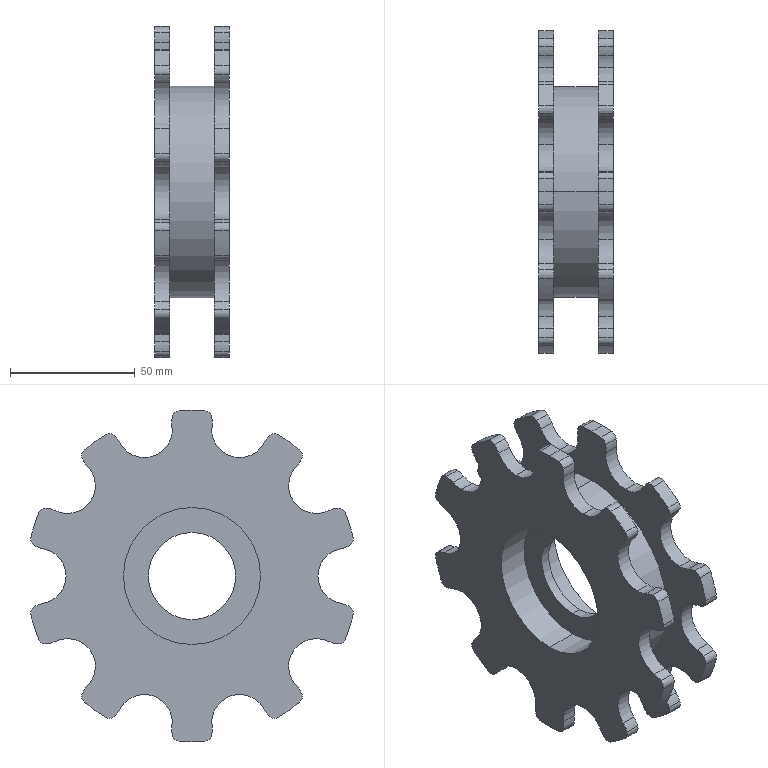Part | STEP file | PN_0005_default | 1 solid | 152 faces | box 30 x 129.474 x 133 mm | volume 166383 mm3 | cylinder 146 | plane 6 | commonest cylinder face diameters 22.23 x68 6 x48 133 x22 55 x4 35 x2 85 x2